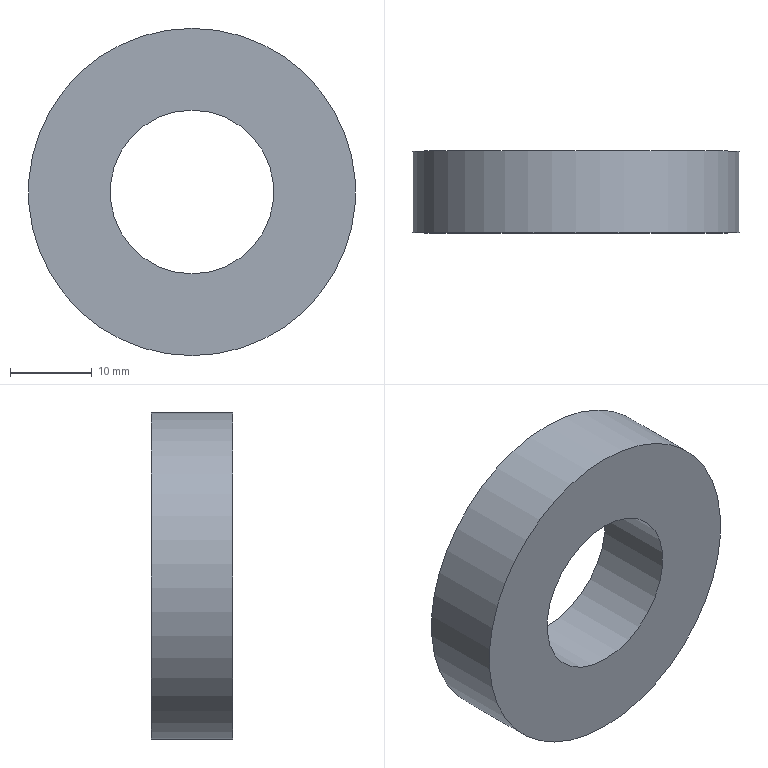Part | STEP file | Fixed ring | 1 solid | 4 faces | box 40 x 10 x 40 mm | volume 9425 mm3 | plane 2 | cylinder 2 | commonest cylinder face diameters 20 x1 40 x1
STEP:
#1=CARTESIAN_POINT('',(0.,10.,20.));
#2=VERTEX_POINT('',#1);
#3=CARTESIAN_POINT('',(0.,10.,0.));
#4=DIRECTION('',(0.,1.,0.));
#5=DIRECTION('',(0.,0.,1.));
#6=AXIS2_PLACEMENT_3D('',#3,#4,#5);
#7=CIRCLE('',#6,20.);
#8=EDGE_CURVE('',#2,#2,#7,.T.);
#9=ORIENTED_EDGE('',*,*,#8,.T.);
#10=EDGE_LOOP('',(#9));
#11=FACE_OUTER_BOUND('',#10,.T.);
#12=CARTESIAN_POINT('',(0.,10.,10.));
#13=VERTEX_POINT('',#12);
#14=CARTESIAN_POINT('',(0.,10.,0.));
#15=DIRECTION('',(0.,1.,0.));
#16=DIRECTION('',(0.,0.,1.));
#17=AXIS2_PLACEMENT_3D('',#14,#15,#16);
#18=CIRCLE('',#17,10.);
#19=EDGE_CURVE('',#13,#13,#18,.T.);
#20=ORIENTED_EDGE('',*,*,#19,.F.);
#21=EDGE_LOOP('',(#20));
#22=FACE_BOUND('',#21,.T.);
#23=CARTESIAN_POINT('',(0.,10.,0.));
#24=DIRECTION('',(0.,1.,0.));
#25=DIRECTION('',(0.,0.,1.));
#26=AXIS2_PLACEMENT_3D('',#23,#24,#25);
#27=PLANE('',#26);
#28=ADVANCED_FACE('',(#11,#22),#27,.T.);
#29=CARTESIAN_POINT('',(0.,0.,20.));
#30=VERTEX_POINT('',#29);
#31=CARTESIAN_POINT('',(0.,0.,0.));
#32=DIRECTION('',(0.,1.,0.));
#33=DIRECTION('',(0.,0.,1.));
#34=AXIS2_PLACEMENT_3D('',#31,#32,#33);
#35=CIRCLE('',#34,20.);
#36=EDGE_CURVE('',#30,#30,#35,.T.);
#37=ORIENTED_EDGE('',*,*,#36,.F.);
#38=EDGE_LOOP('',(#37));
#39=FACE_OUTER_BOUND('',#38,.T.);
#40=CARTESIAN_POINT('',(0.,0.,10.));
#41=VERTEX_POINT('',#40);
#42=CARTESIAN_POINT('',(0.,0.,0.));
#43=DIRECTION('',(0.,1.,0.));
#44=DIRECTION('',(0.,0.,1.));
#45=AXIS2_PLACEMENT_3D('',#42,#43,#44);
#46=CIRCLE('',#45,10.);
#47=EDGE_CURVE('',#41,#41,#46,.T.);
#48=ORIENTED_EDGE('',*,*,#47,.T.);
#49=EDGE_LOOP('',(#48));
#50=FACE_BOUND('',#49,.T.);
#51=CARTESIAN_POINT('',(0.,0.,0.));
#52=DIRECTION('',(0.,1.,0.));
#53=DIRECTION('',(0.,0.,1.));
#54=AXIS2_PLACEMENT_3D('',#51,#52,#53);
#55=PLANE('',#54);
#56=ADVANCED_FACE('',(#39,#50),#55,.F.);
#57=ORIENTED_EDGE('',*,*,#8,.F.);
#58=EDGE_LOOP('',(#57));
#59=FACE_OUTER_BOUND('',#58,.T.);
#60=ORIENTED_EDGE('',*,*,#36,.T.);
#61=EDGE_LOOP('',(#60));
#62=FACE_OUTER_BOUND('',#61,.T.);
#63=CARTESIAN_POINT('',(0.,10.,0.));
#64=DIRECTION('',(0.,-1.,0.));
#65=DIRECTION('',(0.,0.,-1.));
#66=AXIS2_PLACEMENT_3D('',#63,#64,#65);
#67=CYLINDRICAL_SURFACE('',#66,20.);
#68=ADVANCED_FACE('',(#59,#62),#67,.T.);
#69=ORIENTED_EDGE('',*,*,#19,.T.);
#70=EDGE_LOOP('',(#69));
#71=FACE_OUTER_BOUND('',#70,.T.);
#72=ORIENTED_EDGE('',*,*,#47,.F.);
#73=EDGE_LOOP('',(#72));
#74=FACE_OUTER_BOUND('',#73,.T.);
#75=CARTESIAN_POINT('',(0.,10.,0.));
#76=DIRECTION('',(0.,-1.,0.));
#77=DIRECTION('',(0.,0.,-1.));
#78=AXIS2_PLACEMENT_3D('',#75,#76,#77);
#79=CYLINDRICAL_SURFACE('',#78,10.);
#80=ADVANCED_FACE('',(#71,#74),#79,.F.);
#81=CLOSED_SHELL('',(#28,#56,#68,#80));
#82=MANIFOLD_SOLID_BREP('',#81);
#83=CARTESIAN_POINT('',(0.,0.,0.));
#84=DIRECTION('',(0.,0.,1.));
#85=DIRECTION('',(1.,0.,0.));
#86=AXIS2_PLACEMENT_3D('',#83,#84,#85);
#87=(LENGTH_UNIT()NAMED_UNIT(*)SI_UNIT(.MILLI.,.METRE.));
#88=UNCERTAINTY_MEASURE_WITH_UNIT(LENGTH_MEASURE(0.00001),#87,'','');
#89=(NAMED_UNIT(*)PLANE_ANGLE_UNIT()SI_UNIT($,.RADIAN.));
#90=(NAMED_UNIT(*)SI_UNIT($,.STERADIAN.)SOLID_ANGLE_UNIT());
#91=(GEOMETRIC_REPRESENTATION_CONTEXT(3)GLOBAL_UNCERTAINTY_ASSIGNED_CONTEXT((#88))GLOBAL_UNIT_ASSIGNED_CONTEXT((#87,#89,#90))REPRESENTATION_CONTEXT('',''));
#92=ADVANCED_BREP_SHAPE_REPRESENTATION('',(#82,#86),#91);